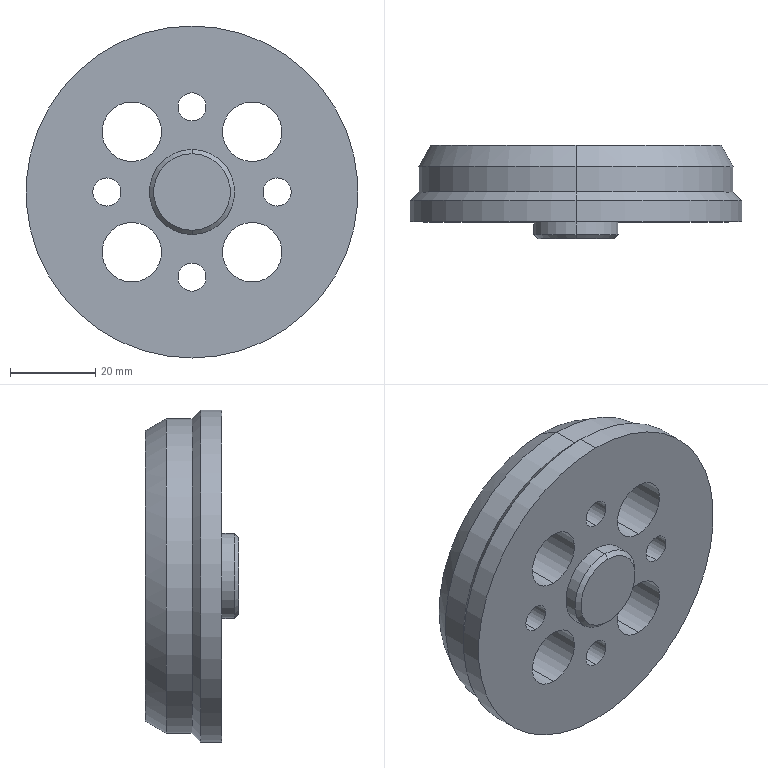Part | STEP file | 0229_215_Holder | 1 solid | 43 faces | box 78 x 22 x 78 mm | volume 64740 mm3 | cylinder 30 | plane 7 | cone 6 | commonest cylinder face diameters 6.6 x8 11 x8 14 x8 20 x2 74 x2 78 x2